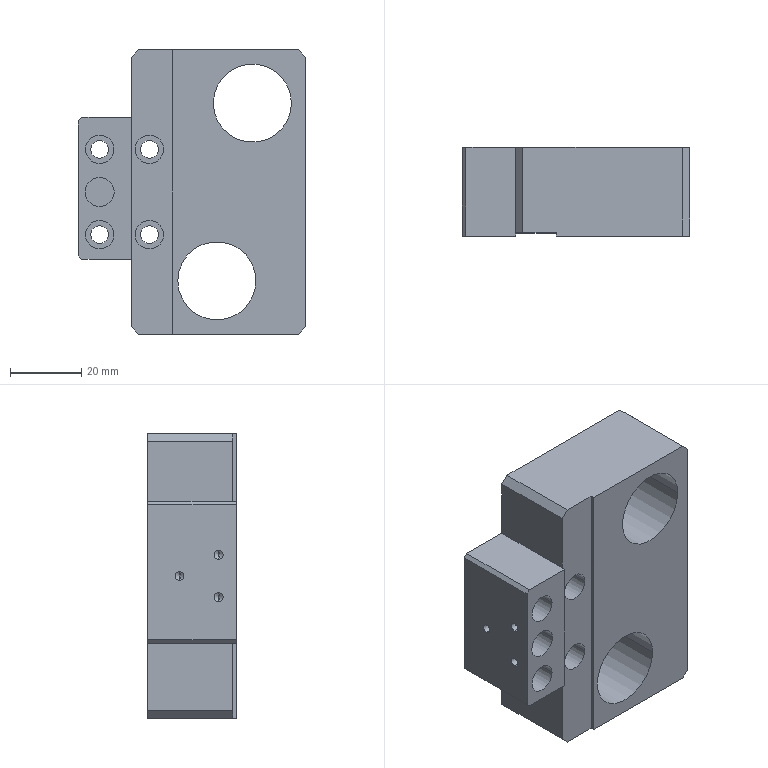Part | SolidWorks | features ICE 6, Chamfer 2, HoleWzd 2, Extrusion 1 | 1 solid | 75 faces | box 64 x 25 x 80 mm | volume 85736 mm3 | cylinder 38 | plane 29 | cone 8 | commonest cylinder face diameters 5 x8 8 x8 2.5 x6 8.2 x6 22 x4 27.5 x4